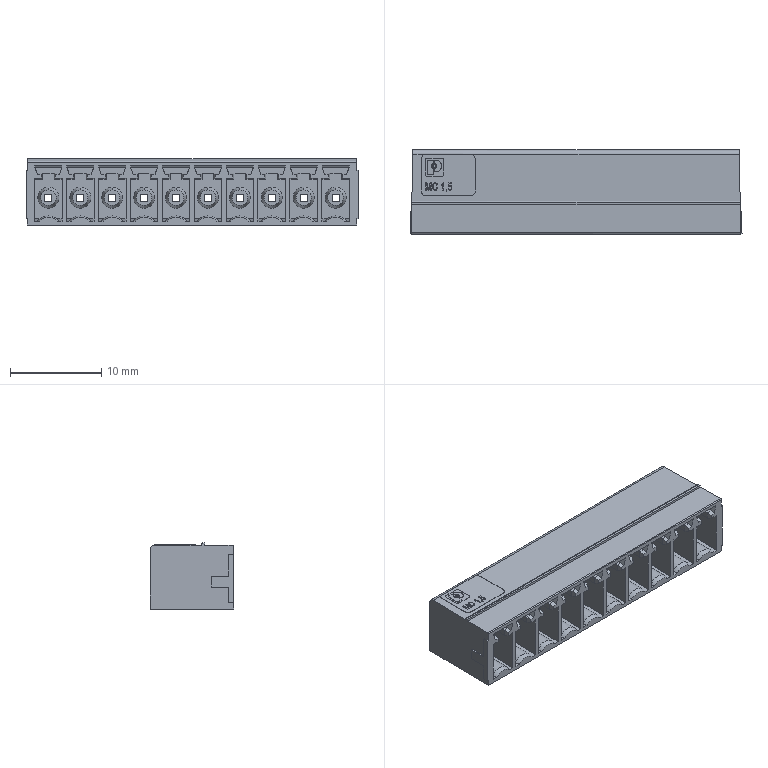Part | STEP file | RJ-USIO-V1_2-220411_239 | 1 solid | 639 faces | box 36.4 x 9.2 x 7.25 mm | volume 1145 mm3 | plane 553 | cylinder 56 | cone 30 | commonest cylinder face diameters 1.25 x20 0.209 x10 3 x10 1 x5 0.278 x4 0.3 x2